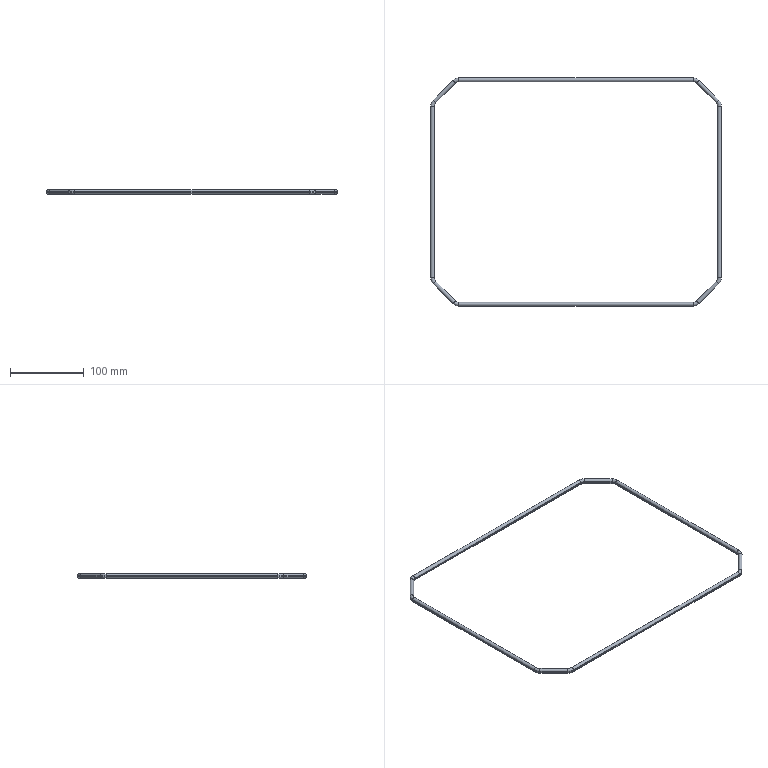Part | SolidWorks | features BaseBody 1 | 1 solid | 128 faces | box 395 x 310 x 6.57 mm | volume 27814 mm3 | cylinder 64 | torus 32 | plane 32 | commonest cylinder face diameters 2 x16 5 x16 13 x8 16 x8 20 x8 23 x8